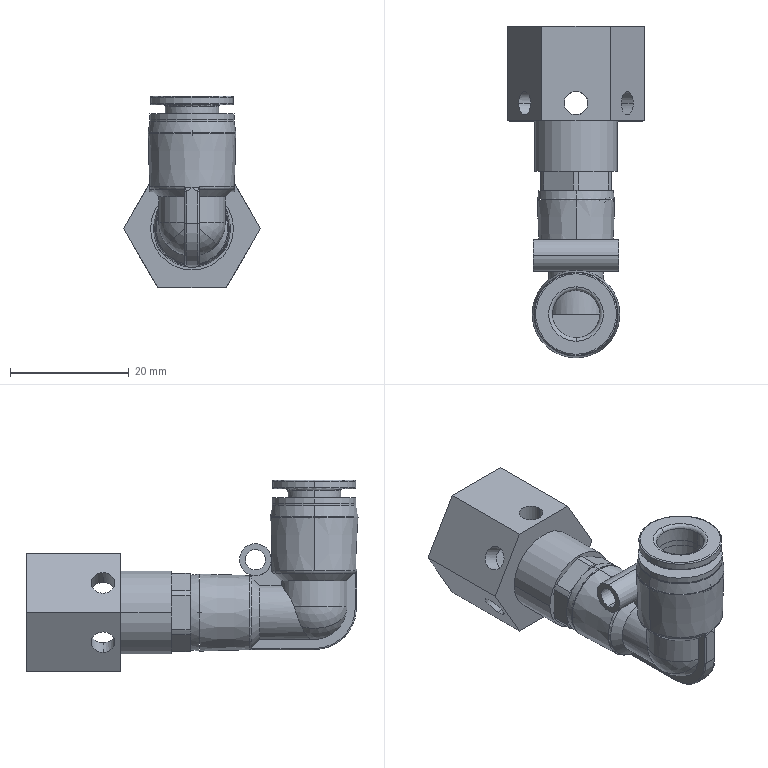Part | SolidWorks | 6 solids | 216 faces | box 23.094 x 55.999 x 32.35 mm | volume 8057 mm3 | cylinder 102 | plane 48 | cone 26 | torus 22 | spline 12 | sphere 6 | commonest cylinder face diameters 8.17 x14 6.779 x13 4 x12 8 x7 8.141 x7 9.85 x7